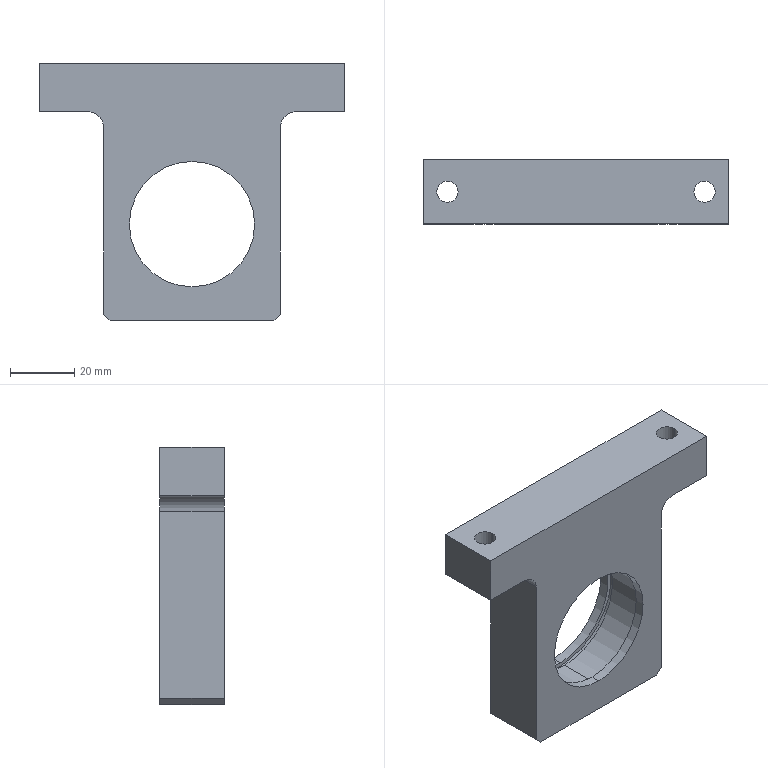Part | SolidWorks | features ICE 2, Chamfer 1, Extrusion 1, Fillet 1, HoleWzd 1 | 1 solid | 29 faces | box 95 x 20 x 80 mm | volume 71658 mm3 | plane 15 | cylinder 14 | commonest cylinder face diameters 6.6 x4 42 x4 10 x2 39 x2 44.5 x2
STEP:
#1=CARTESIAN_POINT('',(0.,16.85,-72.25));
#2=VERTEX_POINT('',#1);
#3=CARTESIAN_POINT('',(0.,16.85,-27.75));
#4=VERTEX_POINT('',#3);
#5=CARTESIAN_POINT('',(0.,16.85,-50.));
#6=DIRECTION('',(0.,1.,0.));
#7=DIRECTION('',(0.,0.,1.));
#8=AXIS2_PLACEMENT_3D('',#5,#6,#7);
#9=CIRCLE('',#8,22.25);
#10=EDGE_CURVE('',#2,#4,#9,.T.);
#11=ORIENTED_EDGE('',*,*,#10,.T.);
#12=CARTESIAN_POINT('',(0.,15.,-27.75));
#13=VERTEX_POINT('',#12);
#14=CARTESIAN_POINT('',(0.,16.85,-27.75));
#15=DIRECTION('',(0.,-1.,0.));
#16=VECTOR('',#15,1000.);
#17=LINE('',#14,#16);
#18=EDGE_CURVE('',#4,#13,#17,.T.);
#19=ORIENTED_EDGE('',*,*,#18,.T.);
#20=CARTESIAN_POINT('',(0.,15.,-72.25));
#21=VERTEX_POINT('',#20);
#22=CARTESIAN_POINT('',(0.,15.,-50.));
#23=DIRECTION('',(0.,1.,0.));
#24=DIRECTION('',(0.,0.,1.));
#25=AXIS2_PLACEMENT_3D('',#22,#23,#24);
#26=CIRCLE('',#25,22.25);
#27=EDGE_CURVE('',#21,#13,#26,.T.);
#28=ORIENTED_EDGE('',*,*,#27,.F.);
#29=CARTESIAN_POINT('',(0.,16.85,-72.25));
#30=DIRECTION('',(0.,-1.,0.));
#31=VECTOR('',#30,1000.);
#32=LINE('',#29,#31);
#33=EDGE_CURVE('',#2,#21,#32,.T.);
#34=ORIENTED_EDGE('',*,*,#33,.F.);
#35=EDGE_LOOP('',(#11,#19,#28,#34));
#36=FACE_OUTER_BOUND('',#35,.T.);
#37=CARTESIAN_POINT('',(0.,16.85,-50.));
#38=DIRECTION('',(0.,-1.,0.));
#39=DIRECTION('',(0.,0.,-1.));
#40=AXIS2_PLACEMENT_3D('',#37,#38,#39);
#41=CYLINDRICAL_SURFACE('',#40,22.25);
#42=ADVANCED_FACE('',(#36),#41,.F.);
#43=CARTESIAN_POINT('',(43.3,10.,0.));
#44=VERTEX_POINT('',#43);
#45=CARTESIAN_POINT('',(36.7,10.,0.));
#46=VERTEX_POINT('',#45);
#47=CARTESIAN_POINT('',(40.,10.,0.));
#48=DIRECTION('',(0.,0.,-1.));
#49=DIRECTION('',(-1.,0.,0.));
#50=AXIS2_PLACEMENT_3D('',#47,#48,#49);
#51=CIRCLE('',#50,3.3);
#52=EDGE_CURVE('',#44,#46,#51,.T.);
#53=ORIENTED_EDGE('',*,*,#52,.F.);
#54=CARTESIAN_POINT('',(43.3,10.,-15.));
#55=VERTEX_POINT('',#54);
#56=CARTESIAN_POINT('',(43.3,10.,-15.));
#57=DIRECTION('',(0.,0.,-1.));
#58=VECTOR('',#57,1000.);
#59=LINE('',#56,#58);
#60=EDGE_CURVE('',#44,#55,#59,.T.);
#61=ORIENTED_EDGE('',*,*,#60,.T.);
#62=CARTESIAN_POINT('',(36.7,10.,-15.));
#63=VERTEX_POINT('',#62);
#64=CARTESIAN_POINT('',(40.,10.,-15.));
#65=DIRECTION('',(0.,0.,-1.));
#66=DIRECTION('',(-1.,0.,0.));
#67=AXIS2_PLACEMENT_3D('',#64,#65,#66);
#68=CIRCLE('',#67,3.3);
#69=EDGE_CURVE('',#55,#63,#68,.T.);
#70=ORIENTED_EDGE('',*,*,#69,.T.);
#71=CARTESIAN_POINT('',(36.7,10.,-15.));
#72=DIRECTION('',(0.,0.,-1.));
#73=VECTOR('',#72,1000.);
#74=LINE('',#71,#73);
#75=EDGE_CURVE('',#46,#63,#74,.T.);
#76=ORIENTED_EDGE('',*,*,#75,.F.);
#77=EDGE_LOOP('',(#53,#61,#70,#76));
#78=FACE_OUTER_BOUND('',#77,.T.);
#79=CARTESIAN_POINT('',(40.,10.,-15.));
#80=DIRECTION('',(0.,0.,-1.));
#81=DIRECTION('',(-1.,0.,0.));
#82=AXIS2_PLACEMENT_3D('',#79,#80,#81);
#83=CYLINDRICAL_SURFACE('',#82,3.3);
#84=ADVANCED_FACE('',(#78),#83,.F.);
#85=CARTESIAN_POINT('',(-36.7,10.,0.));
#86=VERTEX_POINT('',#85);
#87=CARTESIAN_POINT('',(-43.3,10.,0.));
#88=VERTEX_POINT('',#87);
#89=CARTESIAN_POINT('',(-40.,10.,0.));
#90=DIRECTION('',(0.,0.,-1.));
#91=DIRECTION('',(-1.,0.,0.));
#92=AXIS2_PLACEMENT_3D('',#89,#90,#91);
#93=CIRCLE('',#92,3.3);
#94=EDGE_CURVE('',#86,#88,#93,.T.);
#95=ORIENTED_EDGE('',*,*,#94,.F.);
#96=CARTESIAN_POINT('',(-36.7,10.,-15.));
#97=VERTEX_POINT('',#96);
#98=CARTESIAN_POINT('',(-36.7,10.,-15.));
#99=DIRECTION('',(0.,0.,-1.));
#100=VECTOR('',#99,1000.);
#101=LINE('',#98,#100);
#102=EDGE_CURVE('',#86,#97,#101,.T.);
#103=ORIENTED_EDGE('',*,*,#102,.T.);
#104=CARTESIAN_POINT('',(-43.3,10.,-15.));
#105=VERTEX_POINT('',#104);
#106=CARTESIAN_POINT('',(-40.,10.,-15.));
#107=DIRECTION('',(0.,0.,-1.));
#108=DIRECTION('',(-1.,0.,0.));
#109=AXIS2_PLACEMENT_3D('',#106,#107,#108);
#110=CIRCLE('',#109,3.3);
#111=EDGE_CURVE('',#97,#105,#110,.T.);
#112=ORIENTED_EDGE('',*,*,#111,.T.);
#113=CARTESIAN_POINT('',(-43.3,10.,-15.));
#114=DIRECTION('',(0.,0.,-1.));
#115=VECTOR('',#114,1000.);
#116=LINE('',#113,#115);
#117=EDGE_CURVE('',#88,#105,#116,.T.);
#118=ORIENTED_EDGE('',*,*,#117,.F.);
#119=EDGE_LOOP('',(#95,#103,#112,#118));
#120=FACE_OUTER_BOUND('',#119,.T.);
#121=CARTESIAN_POINT('',(-40.,10.,-15.));
#122=DIRECTION('',(0.,0.,-1.));
#123=DIRECTION('',(-1.,0.,0.));
#124=AXIS2_PLACEMENT_3D('',#121,#122,#123);
#125=CYLINDRICAL_SURFACE('',#124,3.3);
#126=ADVANCED_FACE('',(#120),#125,.F.);
#127=CARTESIAN_POINT('',(0.,3.,-30.5));
#128=VERTEX_POINT('',#127);
#129=CARTESIAN_POINT('',(0.,3.,-69.5));
#130=VERTEX_POINT('',#129);
#131=CARTESIAN_POINT('',(0.,3.,-50.));
#132=DIRECTION('',(0.,-1.,0.));
#133=DIRECTION('',(0.,0.,-1.));
#134=AXIS2_PLACEMENT_3D('',#131,#132,#133);
#135=CIRCLE('',#134,19.5);
#136=EDGE_CURVE('',#128,#130,#135,.T.);
#137=ORIENTED_EDGE('',*,*,#136,.F.);
#138=CARTESIAN_POINT('',(0.,0.,-30.5));
#139=VERTEX_POINT('',#138);
#140=CARTESIAN_POINT('',(0.,3.,-30.5));
#141=DIRECTION('',(0.,-1.,0.));
#142=VECTOR('',#141,1000.);
#143=LINE('',#140,#142);
#144=EDGE_CURVE('',#128,#139,#143,.T.);
#145=ORIENTED_EDGE('',*,*,#144,.T.);
#146=CARTESIAN_POINT('',(0.,0.,-69.5));
#147=VERTEX_POINT('',#146);
#148=CARTESIAN_POINT('',(0.,0.,-50.));
#149=DIRECTION('',(0.,-1.,0.));
#150=DIRECTION('',(0.,0.,-1.));
#151=AXIS2_PLACEMENT_3D('',#148,#149,#150);
#152=CIRCLE('',#151,19.5);
#153=EDGE_CURVE('',#139,#147,#152,.T.);
#154=ORIENTED_EDGE('',*,*,#153,.T.);
#155=CARTESIAN_POINT('',(0.,3.,-69.5));
#156=DIRECTION('',(0.,-1.,0.));
#157=VECTOR('',#156,1000.);
#158=LINE('',#155,#157);
#159=EDGE_CURVE('',#130,#147,#158,.T.);
#160=ORIENTED_EDGE('',*,*,#159,.F.);
#161=EDGE_LOOP('',(#137,#145,#154,#160));
#162=FACE_OUTER_BOUND('',#161,.T.);
#163=CARTESIAN_POINT('',(0.,3.,-50.));
#164=DIRECTION('',(0.,-1.,0.));
#165=DIRECTION('',(0.,0.,-1.));
#166=AXIS2_PLACEMENT_3D('',#163,#164,#165);
#167=CYLINDRICAL_SURFACE('',#166,19.5);
#168=ADVANCED_FACE('',(#162),#167,.F.);
#169=CARTESIAN_POINT('',(0.,20.,-71.));
#170=VERTEX_POINT('',#169);
#171=CARTESIAN_POINT('',(0.,20.,-29.));
#172=VERTEX_POINT('',#171);
#173=CARTESIAN_POINT('',(0.,20.,-50.));
#174=DIRECTION('',(0.,1.,0.));
#175=DIRECTION('',(0.,0.,1.));
#176=AXIS2_PLACEMENT_3D('',#173,#174,#175);
#177=CIRCLE('',#176,21.);
#178=EDGE_CURVE('',#170,#172,#177,.T.);
#179=ORIENTED_EDGE('',*,*,#178,.T.);
#180=CARTESIAN_POINT('',(0.,16.85,-29.));
#181=VERTEX_POINT('',#180);
#182=CARTESIAN_POINT('',(0.,20.,-29.));
#183=DIRECTION('',(0.,-1.,0.));
#184=VECTOR('',#183,1000.);
#185=LINE('',#182,#184);
#186=EDGE_CURVE('',#172,#181,#185,.T.);
#187=ORIENTED_EDGE('',*,*,#186,.T.);
#188=CARTESIAN_POINT('',(0.,16.85,-71.));
#189=VERTEX_POINT('',#188);
#190=CARTESIAN_POINT('',(0.,16.85,-50.));
#191=DIRECTION('',(0.,1.,0.));
#192=DIRECTION('',(0.,0.,1.));
#193=AXIS2_PLACEMENT_3D('',#190,#191,#192);
#194=CIRCLE('',#193,21.);
#195=EDGE_CURVE('',#189,#181,#194,.T.);
#196=ORIENTED_EDGE('',*,*,#195,.F.);
#197=CARTESIAN_POINT('',(0.,20.,-71.));
#198=DIRECTION('',(0.,-1.,0.));
#199=VECTOR('',#198,1000.);
#200=LINE('',#197,#199);
#201=EDGE_CURVE('',#170,#189,#200,.T.);
#202=ORIENTED_EDGE('',*,*,#201,.F.);
#203=EDGE_LOOP('',(#179,#187,#196,#202));
#204=FACE_OUTER_BOUND('',#203,.T.);
#205=CARTESIAN_POINT('',(0.,20.,-50.));
#206=DIRECTION('',(0.,-1.,0.));
#207=DIRECTION('',(0.,0.,-1.));
#208=AXIS2_PLACEMENT_3D('',#205,#206,#207);
#209=CYLINDRICAL_SURFACE('',#208,21.);
#210=ADVANCED_FACE('',(#204),#209,.F.);
#211=CARTESIAN_POINT('',(0.,15.,-71.));
#212=VERTEX_POINT('',#211);
#213=CARTESIAN_POINT('',(0.,15.,-29.));
#214=VERTEX_POINT('',#213);
#215=CARTESIAN_POINT('',(0.,15.,-50.));
#216=DIRECTION('',(0.,1.,0.));
#217=DIRECTION('',(0.,0.,1.));
#218=AXIS2_PLACEMENT_3D('',#215,#216,#217);
#219=CIRCLE('',#218,21.);
#220=EDGE_CURVE('',#212,#214,#219,.T.);
#221=ORIENTED_EDGE('',*,*,#220,.T.);
#222=CARTESIAN_POINT('',(0.,3.,-29.));
#223=VERTEX_POINT('',#222);
#224=CARTESIAN_POINT('',(0.,20.,-29.));
#225=DIRECTION('',(0.,-1.,0.));
#226=VECTOR('',#225,1000.);
#227=LINE('',#224,#226);
#228=EDGE_CURVE('',#214,#223,#227,.T.);
#229=ORIENTED_EDGE('',*,*,#228,.T.);
#230=CARTESIAN_POINT('',(0.,3.,-71.));
#231=VERTEX_POINT('',#230);
#232=CARTESIAN_POINT('',(0.,3.,-50.));
#233=DIRECTION('',(0.,-1.,0.));
#234=DIRECTION('',(0.,0.,-1.));
#235=AXIS2_PLACEMENT_3D('',#232,#233,#234);
#236=CIRCLE('',#235,21.);
#237=EDGE_CURVE('',#223,#231,#236,.T.);
#238=ORIENTED_EDGE('',*,*,#237,.T.);
#239=CARTESIAN_POINT('',(0.,20.,-71.));
#240=DIRECTION('',(0.,-1.,0.));
#241=VECTOR('',#240,1000.);
#242=LINE('',#239,#241);
#243=EDGE_CURVE('',#212,#231,#242,.T.);
#244=ORIENTED_EDGE('',*,*,#243,.F.);
#245=EDGE_LOOP('',(#221,#229,#238,#244));
#246=FACE_OUTER_BOUND('',#245,.T.);
#247=CARTESIAN_POINT('',(0.,20.,-50.));
#248=DIRECTION('',(0.,-1.,0.));
#249=DIRECTION('',(0.,0.,-1.));
#250=AXIS2_PLACEMENT_3D('',#247,#248,#249);
#251=CYLINDRICAL_SURFACE('',#250,21.);
#252=ADVANCED_FACE('',(#246),#251,.F.);
#253=ORIENTED_EDGE('',*,*,#228,.F.);
#254=CARTESIAN_POINT('',(0.,15.,-50.));
#255=DIRECTION('',(0.,1.,0.));
#256=DIRECTION('',(0.,0.,1.));
#257=AXIS2_PLACEMENT_3D('',#254,#255,#256);
#258=CIRCLE('',#257,21.);
#259=EDGE_CURVE('',#214,#212,#258,.T.);
#260=ORIENTED_EDGE('',*,*,#259,.T.);
#261=ORIENTED_EDGE('',*,*,#243,.T.);
#262=CARTESIAN_POINT('',(0.,3.,-50.));
#263=DIRECTION('',(0.,-1.,0.));
#264=DIRECTION('',(0.,0.,-1.));
#265=AXIS2_PLACEMENT_3D('',#262,#263,#264);
#266=CIRCLE('',#265,21.);
#267=EDGE_CURVE('',#231,#223,#266,.T.);
#268=ORIENTED_EDGE('',*,*,#267,.T.);
#269=EDGE_LOOP('',(#253,#260,#261,#268));
#270=FACE_OUTER_BOUND('',#269,.T.);
#271=CARTESIAN_POINT('',(0.,20.,-50.));
#272=DIRECTION('',(0.,-1.,0.));
#273=DIRECTION('',(0.,0.,-1.));
#274=AXIS2_PLACEMENT_3D('',#271,#272,#273);
#275=CYLINDRICAL_SURFACE('',#274,21.);
#276=ADVANCED_FACE('',(#270),#275,.F.);
#277=ORIENTED_EDGE('',*,*,#186,.F.);
#278=CARTESIAN_POINT('',(0.,20.,-50.));
#279=DIRECTION('',(0.,1.,0.));
#280=DIRECTION('',(0.,0.,1.));
#281=AXIS2_PLACEMENT_3D('',#278,#279,#280);
#282=CIRCLE('',#281,21.);
#283=EDGE_CURVE('',#172,#170,#282,.T.);
#284=ORIENTED_EDGE('',*,*,#283,.T.);
#285=ORIENTED_EDGE('',*,*,#201,.T.);
#286=CARTESIAN_POINT('',(0.,16.85,-50.));
#287=DIRECTION('',(0.,1.,0.));
#288=DIRECTION('',(0.,0.,1.));
#289=AXIS2_PLACEMENT_3D('',#286,#287,#288);
#290=CIRCLE('',#289,21.);
#291=EDGE_CURVE('',#181,#189,#290,.T.);
#292=ORIENTED_EDGE('',*,*,#291,.F.);
#293=EDGE_LOOP('',(#277,#284,#285,#292));
#294=FACE_OUTER_BOUND('',#293,.T.);
#295=CARTESIAN_POINT('',(0.,20.,-50.));
#296=DIRECTION('',(0.,-1.,0.));
#297=DIRECTION('',(0.,0.,-1.));
#298=AXIS2_PLACEMENT_3D('',#295,#296,#297);
#299=CYLINDRICAL_SURFACE('',#298,21.);
#300=ADVANCED_FACE('',(#294),#299,.F.);
#301=CARTESIAN_POINT('',(47.5,20.,-15.));
#302=VERTEX_POINT('',#301);
#303=CARTESIAN_POINT('',(32.5,20.,-15.));
#304=VERTEX_POINT('',#303);
#305=CARTESIAN_POINT('',(27.5,20.,-15.));
#306=DIRECTION('',(-1.,0.,0.));
#307=VECTOR('',#306,1000.);
#308=LINE('',#305,#307);
#309=EDGE_CURVE('',#302,#304,#308,.T.);
#310=ORIENTED_EDGE('',*,*,#309,.T.);
#311=CARTESIAN_POINT('',(27.5,20.,-20.));
#312=VERTEX_POINT('',#311);
#313=CARTESIAN_POINT('',(32.5,20.,-20.));
#314=DIRECTION('',(0.,-1.,0.));
#315=DIRECTION('',(0.,0.,1.));
#316=AXIS2_PLACEMENT_3D('',#313,#314,#315);
#317=CIRCLE('',#316,5.);
#318=EDGE_CURVE('',#304,#312,#317,.T.);
#319=ORIENTED_EDGE('',*,*,#318,.T.);
#320=CARTESIAN_POINT('',(27.5,20.,-78.));
#321=VERTEX_POINT('',#320);
#322=CARTESIAN_POINT('',(27.5,20.,-80.));
#323=DIRECTION('',(0.,0.,-1.));
#324=VECTOR('',#323,1000.);
#325=LINE('',#322,#324);
#326=EDGE_CURVE('',#312,#321,#325,.T.);
#327=ORIENTED_EDGE('',*,*,#326,.T.);
#328=CARTESIAN_POINT('',(25.5,20.,-80.));
#329=VERTEX_POINT('',#328);
#330=CARTESIAN_POINT('',(52.75,20.,-52.75));
#331=DIRECTION('',(-0.7071,0.,-0.7071));
#332=VECTOR('',#331,1000.);
#333=LINE('',#330,#332);
#334=EDGE_CURVE('',#321,#329,#333,.T.);
#335=ORIENTED_EDGE('',*,*,#334,.T.);
#336=CARTESIAN_POINT('',(-25.5,20.,-80.));
#337=VERTEX_POINT('',#336);
#338=CARTESIAN_POINT('',(-27.5,20.,-80.));
#339=DIRECTION('',(-1.,0.,0.));
#340=VECTOR('',#339,1000.);
#341=LINE('',#338,#340);
#342=EDGE_CURVE('',#329,#337,#341,.T.);
#343=ORIENTED_EDGE('',*,*,#342,.T.);
#344=CARTESIAN_POINT('',(-27.5,20.,-78.));
#345=VERTEX_POINT('',#344);
#346=CARTESIAN_POINT('',(-52.75,20.,-52.75));
#347=DIRECTION('',(-0.7071,0.,0.7071));
#348=VECTOR('',#347,1000.);
#349=LINE('',#346,#348);
#350=EDGE_CURVE('',#337,#345,#349,.T.);
#351=ORIENTED_EDGE('',*,*,#350,.T.);
#352=CARTESIAN_POINT('',(-27.5,20.,-20.));
#353=VERTEX_POINT('',#352);
#354=CARTESIAN_POINT('',(-27.5,20.,-15.));
#355=DIRECTION('',(0.,0.,1.));
#356=VECTOR('',#355,1000.);
#357=LINE('',#354,#356);
#358=EDGE_CURVE('',#345,#353,#357,.T.);
#359=ORIENTED_EDGE('',*,*,#358,.T.);
#360=CARTESIAN_POINT('',(-32.5,20.,-15.));
#361=VERTEX_POINT('',#360);
#362=CARTESIAN_POINT('',(-32.5,20.,-20.));
#363=DIRECTION('',(0.,-1.,0.));
#364=DIRECTION('',(0.,0.,1.));
#365=AXIS2_PLACEMENT_3D('',#362,#363,#364);
#366=CIRCLE('',#365,5.);
#367=EDGE_CURVE('',#353,#361,#366,.T.);
#368=ORIENTED_EDGE('',*,*,#367,.T.);
#369=CARTESIAN_POINT('',(-47.5,20.,-15.));
#370=VERTEX_POINT('',#369);
#371=CARTESIAN_POINT('',(-47.5,20.,-15.));
#372=DIRECTION('',(-1.,0.,0.));
#373=VECTOR('',#372,1000.);
#374=LINE('',#371,#373);
#375=EDGE_CURVE('',#361,#370,#374,.T.);
#376=ORIENTED_EDGE('',*,*,#375,.T.);
#377=CARTESIAN_POINT('',(-47.5,20.,0.));
#378=VERTEX_POINT('',#377);
#379=CARTESIAN_POINT('',(-47.5,20.,0.));
#380=DIRECTION('',(0.,0.,1.));
#381=VECTOR('',#380,1000.);
#382=LINE('',#379,#381);
#383=EDGE_CURVE('',#370,#378,#382,.T.);
#384=ORIENTED_EDGE('',*,*,#383,.T.);
#385=CARTESIAN_POINT('',(47.5,20.,0.));
#386=VERTEX_POINT('',#385);
#387=CARTESIAN_POINT('',(-47.5,20.,0.));
#388=DIRECTION('',(1.,0.,0.));
#389=VECTOR('',#388,1000.);
#390=LINE('',#387,#389);
#391=EDGE_CURVE('',#378,#386,#390,.T.);
#392=ORIENTED_EDGE('',*,*,#391,.T.);
#393=CARTESIAN_POINT('',(47.5,20.,-15.));
#394=DIRECTION('',(0.,0.,-1.));
#395=VECTOR('',#394,1000.);
#396=LINE('',#393,#395);
#397=EDGE_CURVE('',#386,#302,#396,.T.);
#398=ORIENTED_EDGE('',*,*,#397,.T.);
#399=EDGE_LOOP('',(#310,#319,#327,#335,#343,#351,#359,#368,#376,#384,#392,#398));
#400=FACE_OUTER_BOUND('',#399,.T.);
#401=ORIENTED_EDGE('',*,*,#178,.F.);
#402=ORIENTED_EDGE('',*,*,#283,.F.);
#403=EDGE_LOOP('',(#401,#402));
#404=FACE_BOUND('',#403,.T.);
#405=CARTESIAN_POINT('',(0.,20.,0.));
#406=DIRECTION('',(0.,1.,0.));
#407=DIRECTION('',(0.,0.,1.));
#408=AXIS2_PLACEMENT_3D('',#405,#406,#407);
#409=PLANE('',#408);
#410=ADVANCED_FACE('',(#400,#404),#409,.T.);
#411=CARTESIAN_POINT('',(25.5,0.,-80.));
#412=VERTEX_POINT('',#411);
#413=CARTESIAN_POINT('',(-25.5,0.,-80.));
#414=VERTEX_POINT('',#413);
#415=CARTESIAN_POINT('',(-27.5,0.,-80.));
#416=DIRECTION('',(-1.,0.,0.));
#417=VECTOR('',#416,1000.);
#418=LINE('',#415,#417);
#419=EDGE_CURVE('',#412,#414,#418,.T.);
#420=ORIENTED_EDGE('',*,*,#419,.F.);
#421=CARTESIAN_POINT('',(27.5,0.,-78.));
#422=VERTEX_POINT('',#421);
#423=CARTESIAN_POINT('',(25.5,0.,-80.));
#424=DIRECTION('',(0.7071,0.,0.7071));
#425=VECTOR('',#424,1000.);
#426=LINE('',#423,#425);
#427=EDGE_CURVE('',#412,#422,#426,.T.);
#428=ORIENTED_EDGE('',*,*,#427,.T.);
#429=CARTESIAN_POINT('',(27.5,0.,-20.));
#430=VERTEX_POINT('',#429);
#431=CARTESIAN_POINT('',(27.5,0.,-80.));
#432=DIRECTION('',(0.,0.,-1.));
#433=VECTOR('',#432,1000.);
#434=LINE('',#431,#433);
#435=EDGE_CURVE('',#430,#422,#434,.T.);
#436=ORIENTED_EDGE('',*,*,#435,.F.);
#437=CARTESIAN_POINT('',(32.5,0.,-15.));
#438=VERTEX_POINT('',#437);
#439=CARTESIAN_POINT('',(32.5,0.,-20.));
#440=DIRECTION('',(0.,1.,0.));
#441=DIRECTION('',(0.,0.,1.));
#442=AXIS2_PLACEMENT_3D('',#439,#440,#441);
#443=CIRCLE('',#442,5.);
#444=EDGE_CURVE('',#430,#438,#443,.T.);
#445=ORIENTED_EDGE('',*,*,#444,.T.);
#446=CARTESIAN_POINT('',(47.5,0.,-15.));
#447=VERTEX_POINT('',#446);
#448=CARTESIAN_POINT('',(27.5,0.,-15.));
#449=DIRECTION('',(-1.,0.,0.));
#450=VECTOR('',#449,1000.);
#451=LINE('',#448,#450);
#452=EDGE_CURVE('',#447,#438,#451,.T.);
#453=ORIENTED_EDGE('',*,*,#452,.F.);
#454=CARTESIAN_POINT('',(47.5,0.,0.));
#455=VERTEX_POINT('',#454);
#456=CARTESIAN_POINT('',(47.5,0.,-15.));
#457=DIRECTION('',(0.,0.,-1.));
#458=VECTOR('',#457,1000.);
#459=LINE('',#456,#458);
#460=EDGE_CURVE('',#455,#447,#459,.T.);
#461=ORIENTED_EDGE('',*,*,#460,.F.);
#462=CARTESIAN_POINT('',(-47.5,0.,0.));
#463=VERTEX_POINT('',#462);
#464=CARTESIAN_POINT('',(-47.5,0.,0.));
#465=DIRECTION('',(1.,0.,0.));
#466=VECTOR('',#465,1000.);
#467=LINE('',#464,#466);
#468=EDGE_CURVE('',#463,#455,#467,.T.);
#469=ORIENTED_EDGE('',*,*,#468,.F.);
#470=CARTESIAN_POINT('',(-47.5,0.,-15.));
#471=VERTEX_POINT('',#470);
#472=CARTESIAN_POINT('',(-47.5,0.,0.));
#473=DIRECTION('',(0.,0.,1.));
#474=VECTOR('',#473,1000.);
#475=LINE('',#472,#474);
#476=EDGE_CURVE('',#471,#463,#475,.T.);
#477=ORIENTED_EDGE('',*,*,#476,.F.);
#478=CARTESIAN_POINT('',(-32.5,0.,-15.));
#479=VERTEX_POINT('',#478);
#480=CARTESIAN_POINT('',(-47.5,0.,-15.));
#481=DIRECTION('',(-1.,0.,0.));
#482=VECTOR('',#481,1000.);
#483=LINE('',#480,#482);
#484=EDGE_CURVE('',#479,#471,#483,.T.);
#485=ORIENTED_EDGE('',*,*,#484,.F.);
#486=CARTESIAN_POINT('',(-27.5,0.,-20.));
#487=VERTEX_POINT('',#486);
#488=CARTESIAN_POINT('',(-32.5,0.,-20.));
#489=DIRECTION('',(0.,1.,0.));
#490=DIRECTION('',(0.,0.,1.));
#491=AXIS2_PLACEMENT_3D('',#488,#489,#490);
#492=CIRCLE('',#491,5.);
#493=EDGE_CURVE('',#479,#487,#492,.T.);
#494=ORIENTED_EDGE('',*,*,#493,.T.);
#495=CARTESIAN_POINT('',(-27.5,0.,-78.));
#496=VERTEX_POINT('',#495);
#497=CARTESIAN_POINT('',(-27.5,0.,-15.));
#498=DIRECTION('',(0.,0.,1.));
#499=VECTOR('',#498,1000.);
#500=LINE('',#497,#499);
#501=EDGE_CURVE('',#496,#487,#500,.T.);
#502=ORIENTED_EDGE('',*,*,#501,.F.);
#503=CARTESIAN_POINT('',(-27.5,0.,-78.));
#504=DIRECTION('',(0.7071,0.,-0.7071));
#505=VECTOR('',#504,1000.);
#506=LINE('',#503,#505);
#507=EDGE_CURVE('',#496,#414,#506,.T.);
#508=ORIENTED_EDGE('',*,*,#507,.T.);
#509=EDGE_LOOP('',(#420,#428,#436,#445,#453,#461,#469,#477,#485,#494,#502,#508));
#510=FACE_OUTER_BOUND('',#509,.T.);
#511=CARTESIAN_POINT('',(0.,0.,-50.));
#512=DIRECTION('',(0.,-1.,0.));
#513=DIRECTION('',(0.,0.,-1.));
#514=AXIS2_PLACEMENT_3D('',#511,#512,#513);
#515=CIRCLE('',#514,19.5);
#516=EDGE_CURVE('',#147,#139,#515,.T.);
#517=ORIENTED_EDGE('',*,*,#516,.F.);
#518=ORIENTED_EDGE('',*,*,#153,.F.);
#519=EDGE_LOOP('',(#517,#518));
#520=FACE_BOUND('',#519,.T.);
#521=CARTESIAN_POINT('',(0.,0.,0.));
#522=DIRECTION('',(0.,1.,0.));
#523=DIRECTION('',(0.,0.,1.));
#524=AXIS2_PLACEMENT_3D('',#521,#522,#523);
#525=PLANE('',#524);
#526=ADVANCED_FACE('',(#510,#520),#525,.F.);
#527=ORIENTED_EDGE('',*,*,#460,.T.);
#528=CARTESIAN_POINT('',(47.5,20.,-15.));
#529=DIRECTION('',(0.,-1.,0.));
#530=VECTOR('',#529,1000.);
#531=LINE('',#528,#530);
#532=EDGE_CURVE('',#302,#447,#531,.T.);
#533=ORIENTED_EDGE('',*,*,#532,.F.);
#534=ORIENTED_EDGE('',*,*,#397,.F.);
#535=CARTESIAN_POINT('',(47.5,20.,0.));
#536=DIRECTION('',(0.,-1.,0.));
#537=VECTOR('',#536,1000.);
#538=LINE('',#535,#537);
#539=EDGE_CURVE('',#386,#455,#538,.T.);
#540=ORIENTED_EDGE('',*,*,#539,.T.);
#541=EDGE_LOOP('',(#527,#533,#534,#540));
#542=FACE_OUTER_BOUND('',#541,.T.);
#543=CARTESIAN_POINT('',(47.5,20.,-15.));
#544=DIRECTION('',(-1.,0.,0.));
#545=DIRECTION('',(0.,0.,1.));
#546=AXIS2_PLACEMENT_3D('',#543,#544,#545);
#547=PLANE('',#546);
#548=ADVANCED_FACE('',(#542),#547,.F.);
#549=CARTESIAN_POINT('',(40.,10.,-15.));
#550=DIRECTION('',(0.,0.,-1.));
#551=DIRECTION('',(-1.,0.,0.));
#552=AXIS2_PLACEMENT_3D('',#549,#550,#551);
#553=CIRCLE('',#552,3.3);
#554=EDGE_CURVE('',#63,#55,#553,.T.);
#555=ORIENTED_EDGE('',*,*,#554,.F.);
#556=ORIENTED_EDGE('',*,*,#69,.F.);
#557=EDGE_LOOP('',(#555,#556));
#558=FACE_BOUND('',#557,.T.);
#559=ORIENTED_EDGE('',*,*,#452,.T.);
#560=CARTESIAN_POINT('',(32.5,20.,-15.));
#561=DIRECTION('',(0.,1.,0.));
#562=VECTOR('',#561,1000.);
#563=LINE('',#560,#562);
#564=EDGE_CURVE('',#438,#304,#563,.T.);
#565=ORIENTED_EDGE('',*,*,#564,.T.);
#566=ORIENTED_EDGE('',*,*,#309,.F.);
#567=ORIENTED_EDGE('',*,*,#532,.T.);
#568=EDGE_LOOP('',(#559,#565,#566,#567));
#569=FACE_OUTER_BOUND('',#568,.T.);
#570=CARTESIAN_POINT('',(27.5,20.,-15.));
#571=DIRECTION('',(0.,0.,1.));
#572=DIRECTION('',(1.,0.,0.));
#573=AXIS2_PLACEMENT_3D('',#570,#571,#572);
#574=PLANE('',#573);
#575=ADVANCED_FACE('',(#558,#569),#574,.F.);
#576=ORIENTED_EDGE('',*,*,#326,.F.);
#577=CARTESIAN_POINT('',(27.5,0.,-20.));
#578=DIRECTION('',(0.,-1.,0.));
#579=VECTOR('',#578,1000.);
#580=LINE('',#577,#579);
#581=EDGE_CURVE('',#312,#430,#580,.T.);
#582=ORIENTED_EDGE('',*,*,#581,.T.);
#583=ORIENTED_EDGE('',*,*,#435,.T.);
#584=CARTESIAN_POINT('',(27.5,20.,-78.));
#585=DIRECTION('',(0.,1.,0.));
#586=VECTOR('',#585,1000.);
#587=LINE('',#584,#586);
#588=EDGE_CURVE('',#422,#321,#587,.T.);
#589=ORIENTED_EDGE('',*,*,#588,.T.);
#590=EDGE_LOOP('',(#576,#582,#583,#589));
#591=FACE_OUTER_BOUND('',#590,.T.);
#592=CARTESIAN_POINT('',(27.5,20.,-80.));
#593=DIRECTION('',(-1.,0.,0.));
#594=DIRECTION('',(0.,0.,1.));
#595=AXIS2_PLACEMENT_3D('',#592,#593,#594);
#596=PLANE('',#595);
#597=ADVANCED_FACE('',(#591),#596,.F.);
#598=ORIENTED_EDGE('',*,*,#342,.F.);
#599=CARTESIAN_POINT('',(25.5,20.,-80.));
#600=DIRECTION('',(0.,-1.,0.));
#601=VECTOR('',#600,1000.);
#602=LINE('',#599,#601);
#603=EDGE_CURVE('',#329,#412,#602,.T.);
#604=ORIENTED_EDGE('',*,*,#603,.T.);
#605=ORIENTED_EDGE('',*,*,#419,.T.);
#606=CARTESIAN_POINT('',(-25.5,20.,-80.));
#607=DIRECTION('',(0.,1.,0.));
#608=VECTOR('',#607,1000.);
#609=LINE('',#606,#608);
#610=EDGE_CURVE('',#414,#337,#609,.T.);
#611=ORIENTED_EDGE('',*,*,#610,.T.);
#612=EDGE_LOOP('',(#598,#604,#605,#611));
#613=FACE_OUTER_BOUND('',#612,.T.);
#614=CARTESIAN_POINT('',(-27.5,20.,-80.));
#615=DIRECTION('',(0.,0.,1.));
#616=DIRECTION('',(1.,0.,0.));
#617=AXIS2_PLACEMENT_3D('',#614,#615,#616);
#618=PLANE('',#617);
#619=ADVANCED_FACE('',(#613),#618,.F.);
#620=ORIENTED_EDGE('',*,*,#501,.T.);
#621=CARTESIAN_POINT('',(-27.5,20.,-20.));
#622=DIRECTION('',(0.,1.,0.));
#623=VECTOR('',#622,1000.);
#624=LINE('',#621,#623);
#625=EDGE_CURVE('',#487,#353,#624,.T.);
#626=ORIENTED_EDGE('',*,*,#625,.T.);
#627=ORIENTED_EDGE('',*,*,#358,.F.);
#628=CARTESIAN_POINT('',(-27.5,20.,-78.));
#629=DIRECTION('',(0.,-1.,0.));
#630=VECTOR('',#629,1000.);
#631=LINE('',#628,#630);
#632=EDGE_CURVE('',#345,#496,#631,.T.);
#633=ORIENTED_EDGE('',*,*,#632,.T.);
#634=EDGE_LOOP('',(#620,#626,#627,#633));
#635=FACE_OUTER_BOUND('',#634,.T.);
#636=CARTESIAN_POINT('',(-27.5,20.,-15.));
#637=DIRECTION('',(1.,0.,0.));
#638=DIRECTION('',(0.,0.,-1.));
#639=AXIS2_PLACEMENT_3D('',#636,#637,#638);
#640=PLANE('',#639);
#641=ADVANCED_FACE('',(#635),#640,.F.);
#642=CARTESIAN_POINT('',(-40.,10.,-15.));
#643=DIRECTION('',(0.,0.,-1.));
#644=DIRECTION('',(-1.,0.,0.));
#645=AXIS2_PLACEMENT_3D('',#642,#643,#644);
#646=CIRCLE('',#645,3.3);
#647=EDGE_CURVE('',#105,#97,#646,.T.);
#648=ORIENTED_EDGE('',*,*,#647,.F.);
#649=ORIENTED_EDGE('',*,*,#111,.F.);
#650=EDGE_LOOP('',(#648,#649));
#651=FACE_BOUND('',#650,.T.);
#652=ORIENTED_EDGE('',*,*,#375,.F.);
#653=CARTESIAN_POINT('',(-32.5,0.,-15.));
#654=DIRECTION('',(0.,-1.,0.));
#655=VECTOR('',#654,1000.);
#656=LINE('',#653,#655);
#657=EDGE_CURVE('',#361,#479,#656,.T.);
#658=ORIENTED_EDGE('',*,*,#657,.T.);
#659=ORIENTED_EDGE('',*,*,#484,.T.);
#660=CARTESIAN_POINT('',(-47.5,20.,-15.));
#661=DIRECTION('',(0.,-1.,0.));
#662=VECTOR('',#661,1000.);
#663=LINE('',#660,#662);
#664=EDGE_CURVE('',#370,#471,#663,.T.);
#665=ORIENTED_EDGE('',*,*,#664,.F.);
#666=EDGE_LOOP('',(#652,#658,#659,#665));
#667=FACE_OUTER_BOUND('',#666,.T.);
#668=CARTESIAN_POINT('',(-47.5,20.,-15.));
#669=DIRECTION('',(0.,0.,1.));
#670=DIRECTION('',(1.,0.,0.));
#671=AXIS2_PLACEMENT_3D('',#668,#669,#670);
#672=PLANE('',#671);
#673=ADVANCED_FACE('',(#651,#667),#672,.F.);
#674=ORIENTED_EDGE('',*,*,#476,.T.);
#675=CARTESIAN_POINT('',(-47.5,20.,0.));
#676=DIRECTION('',(0.,-1.,0.));
#677=VECTOR('',#676,1000.);
#678=LINE('',#675,#677);
#679=EDGE_CURVE('',#378,#463,#678,.T.);
#680=ORIENTED_EDGE('',*,*,#679,.F.);
#681=ORIENTED_EDGE('',*,*,#383,.F.);
#682=ORIENTED_EDGE('',*,*,#664,.T.);
#683=EDGE_LOOP('',(#674,#680,#681,#682));
#684=FACE_OUTER_BOUND('',#683,.T.);
#685=CARTESIAN_POINT('',(-47.5,20.,0.));
#686=DIRECTION('',(1.,0.,0.));
#687=DIRECTION('',(0.,0.,-1.));
#688=AXIS2_PLACEMENT_3D('',#685,#686,#687);
#689=PLANE('',#688);
#690=ADVANCED_FACE('',(#684),#689,.F.);
#691=CARTESIAN_POINT('',(40.,10.,0.));
#692=DIRECTION('',(0.,0.,-1.));
#693=DIRECTION('',(-1.,0.,0.));
#694=AXIS2_PLACEMENT_3D('',#691,#692,#693);
#695=CIRCLE('',#694,3.3);
#696=EDGE_CURVE('',#46,#44,#695,.T.);
#697=ORIENTED_EDGE('',*,*,#696,.T.);
#698=ORIENTED_EDGE('',*,*,#52,.T.);
#699=EDGE_LOOP('',(#697,#698));
#700=FACE_BOUND('',#699,.T.);
#701=CARTESIAN_POINT('',(-40.,10.,0.));
#702=DIRECTION('',(0.,0.,-1.));
#703=DIRECTION('',(-1.,0.,0.));
#704=AXIS2_PLACEMENT_3D('',#701,#702,#703);
#705=CIRCLE('',#704,3.3);
#706=EDGE_CURVE('',#88,#86,#705,.T.);
#707=ORIENTED_EDGE('',*,*,#706,.T.);
#708=ORIENTED_EDGE('',*,*,#94,.T.);
#709=EDGE_LOOP('',(#707,#708));
#710=FACE_BOUND('',#709,.T.);
#711=ORIENTED_EDGE('',*,*,#468,.T.);
#712=ORIENTED_EDGE('',*,*,#539,.F.);
#713=ORIENTED_EDGE('',*,*,#391,.F.);
#714=ORIENTED_EDGE('',*,*,#679,.T.);
#715=EDGE_LOOP('',(#711,#712,#713,#714));
#716=FACE_OUTER_BOUND('',#715,.T.);
#717=CARTESIAN_POINT('',(-47.5,20.,0.));
#718=DIRECTION('',(0.,0.,-1.));
#719=DIRECTION('',(-1.,0.,0.));
#720=AXIS2_PLACEMENT_3D('',#717,#718,#719);
#721=PLANE('',#720);
#722=ADVANCED_FACE('',(#700,#710,#716),#721,.F.);
#723=ORIENTED_EDGE('',*,*,#334,.F.);
#724=ORIENTED_EDGE('',*,*,#588,.F.);
#725=ORIENTED_EDGE('',*,*,#427,.F.);
#726=ORIENTED_EDGE('',*,*,#603,.F.);
#727=EDGE_LOOP('',(#723,#724,#725,#726));
#728=FACE_OUTER_BOUND('',#727,.T.);
#729=CARTESIAN_POINT('',(25.5,20.,-80.));
#730=DIRECTION('',(-0.7071,0.,0.7071));
#731=DIRECTION('',(0.,-1.,0.));
#732=AXIS2_PLACEMENT_3D('',#729,#730,#731);
#733=PLANE('',#732);
#734=ADVANCED_FACE('',(#728),#733,.F.);
#735=ORIENTED_EDGE('',*,*,#350,.F.);
#736=ORIENTED_EDGE('',*,*,#610,.F.);
#737=ORIENTED_EDGE('',*,*,#507,.F.);
#738=ORIENTED_EDGE('',*,*,#632,.F.);
#739=EDGE_LOOP('',(#735,#736,#737,#738));
#740=FACE_OUTER_BOUND('',#739,.T.);
#741=CARTESIAN_POINT('',(-27.5,20.,-78.));
#742=DIRECTION('',(0.7071,0.,0.7071));
#743=DIRECTION('',(0.,-1.,0.));
#744=AXIS2_PLACEMENT_3D('',#741,#742,#743);
#745=PLANE('',#744);
#746=ADVANCED_FACE('',(#740),#745,.F.);
#747=ORIENTED_EDGE('',*,*,#318,.F.);
#748=ORIENTED_EDGE('',*,*,#564,.F.);
#749=ORIENTED_EDGE('',*,*,#444,.F.);
#750=ORIENTED_EDGE('',*,*,#581,.F.);
#751=EDGE_LOOP('',(#747,#748,#749,#750));
#752=FACE_OUTER_BOUND('',#751,.T.);
#753=CARTESIAN_POINT('',(32.5,20.,-20.));
#754=DIRECTION('',(0.,1.,0.));
#755=DIRECTION('',(0.,0.,1.));
#756=AXIS2_PLACEMENT_3D('',#753,#754,#755);
#757=CYLINDRICAL_SURFACE('',#756,5.);
#758=ADVANCED_FACE('',(#752),#757,.F.);
#759=ORIENTED_EDGE('',*,*,#367,.F.);
#760=ORIENTED_EDGE('',*,*,#625,.F.);
#761=ORIENTED_EDGE('',*,*,#493,.F.);
#762=ORIENTED_EDGE('',*,*,#657,.F.);
#763=EDGE_LOOP('',(#759,#760,#761,#762));
#764=FACE_OUTER_BOUND('',#763,.T.);
#765=CARTESIAN_POINT('',(-32.5,20.,-20.));
#766=DIRECTION('',(0.,1.,0.));
#767=DIRECTION('',(0.,0.,1.));
#768=AXIS2_PLACEMENT_3D('',#765,#766,#767);
#769=CYLINDRICAL_SURFACE('',#768,5.);
#770=ADVANCED_FACE('',(#764),#769,.F.);
#771=CARTESIAN_POINT('',(0.,3.,-50.));
#772=DIRECTION('',(0.,-1.,0.));
#773=DIRECTION('',(0.,0.,-1.));
#774=AXIS2_PLACEMENT_3D('',#771,#772,#773);
#775=CIRCLE('',#774,19.5);
#776=EDGE_CURVE('',#130,#128,#775,.T.);
#777=ORIENTED_EDGE('',*,*,#776,.T.);
#778=ORIENTED_EDGE('',*,*,#136,.T.);
#779=EDGE_LOOP('',(#777,#778));
#780=FACE_BOUND('',#779,.T.);
#781=ORIENTED_EDGE('',*,*,#267,.F.);
#782=ORIENTED_EDGE('',*,*,#237,.F.);
#783=EDGE_LOOP('',(#781,#782));
#784=FACE_OUTER_BOUND('',#783,.T.);
#785=CARTESIAN_POINT('',(0.,3.,-50.));
#786=DIRECTION('',(0.,-1.,0.));
#787=DIRECTION('',(0.,0.,-1.));
#788=AXIS2_PLACEMENT_3D('',#785,#786,#787);
#789=PLANE('',#788);
#790=ADVANCED_FACE('',(#780,#784),#789,.F.);
#791=ORIENTED_EDGE('',*,*,#144,.F.);
#792=ORIENTED_EDGE('',*,*,#776,.F.);
#793=ORIENTED_EDGE('',*,*,#159,.T.);
#794=ORIENTED_EDGE('',*,*,#516,.T.);
#795=EDGE_LOOP('',(#791,#792,#793,#794));
#796=FACE_OUTER_BOUND('',#795,.T.);
#797=CARTESIAN_POINT('',(0.,3.,-50.));
#798=DIRECTION('',(0.,-1.,0.));
#799=DIRECTION('',(0.,0.,-1.));
#800=AXIS2_PLACEMENT_3D('',#797,#798,#799);
#801=CYLINDRICAL_SURFACE('',#800,19.5);
#802=ADVANCED_FACE('',(#796),#801,.F.);
#803=ORIENTED_EDGE('',*,*,#102,.F.);
#804=ORIENTED_EDGE('',*,*,#706,.F.);
#805=ORIENTED_EDGE('',*,*,#117,.T.);
#806=ORIENTED_EDGE('',*,*,#647,.T.);
#807=EDGE_LOOP('',(#803,#804,#805,#806));
#808=FACE_OUTER_BOUND('',#807,.T.);
#809=CARTESIAN_POINT('',(-40.,10.,-15.));
#810=DIRECTION('',(0.,0.,-1.));
#811=DIRECTION('',(-1.,0.,0.));
#812=AXIS2_PLACEMENT_3D('',#809,#810,#811);
#813=CYLINDRICAL_SURFACE('',#812,3.3);
#814=ADVANCED_FACE('',(#808),#813,.F.);
#815=ORIENTED_EDGE('',*,*,#60,.F.);
#816=ORIENTED_EDGE('',*,*,#696,.F.);
#817=ORIENTED_EDGE('',*,*,#75,.T.);
#818=ORIENTED_EDGE('',*,*,#554,.T.);
#819=EDGE_LOOP('',(#815,#816,#817,#818));
#820=FACE_OUTER_BOUND('',#819,.T.);
#821=CARTESIAN_POINT('',(40.,10.,-15.));
#822=DIRECTION('',(0.,0.,-1.));
#823=DIRECTION('',(-1.,0.,0.));
#824=AXIS2_PLACEMENT_3D('',#821,#822,#823);
#825=CYLINDRICAL_SURFACE('',#824,3.3);
#826=ADVANCED_FACE('',(#820),#825,.F.);
#827=ORIENTED_EDGE('',*,*,#10,.F.);
#828=CARTESIAN_POINT('',(0.,16.85,-50.));
#829=DIRECTION('',(0.,1.,0.));
#830=DIRECTION('',(0.,0.,1.));
#831=AXIS2_PLACEMENT_3D('',#828,#829,#830);
#832=CIRCLE('',#831,22.25);
#833=EDGE_CURVE('',#4,#2,#832,.T.);
#834=ORIENTED_EDGE('',*,*,#833,.F.);
#835=EDGE_LOOP('',(#827,#834));
#836=FACE_OUTER_BOUND('',#835,.T.);
#837=ORIENTED_EDGE('',*,*,#195,.T.);
#838=ORIENTED_EDGE('',*,*,#291,.T.);
#839=EDGE_LOOP('',(#837,#838));
#840=FACE_BOUND('',#839,.T.);
#841=CARTESIAN_POINT('',(0.,16.85,-50.));
#842=DIRECTION('',(0.,1.,0.));
#843=DIRECTION('',(0.,0.,1.));
#844=AXIS2_PLACEMENT_3D('',#841,#842,#843);
#845=PLANE('',#844);
#846=ADVANCED_FACE('',(#836,#840),#845,.F.);
#847=ORIENTED_EDGE('',*,*,#27,.T.);
#848=CARTESIAN_POINT('',(0.,15.,-50.));
#849=DIRECTION('',(0.,1.,0.));
#850=DIRECTION('',(0.,0.,1.));
#851=AXIS2_PLACEMENT_3D('',#848,#849,#850);
#852=CIRCLE('',#851,22.25);
#853=EDGE_CURVE('',#13,#21,#852,.T.);
#854=ORIENTED_EDGE('',*,*,#853,.T.);
#855=EDGE_LOOP('',(#847,#854));
#856=FACE_OUTER_BOUND('',#855,.T.);
#857=ORIENTED_EDGE('',*,*,#220,.F.);
#858=ORIENTED_EDGE('',*,*,#259,.F.);
#859=EDGE_LOOP('',(#857,#858));
#860=FACE_BOUND('',#859,.T.);
#861=CARTESIAN_POINT('',(0.,15.,-50.));
#862=DIRECTION('',(0.,1.,0.));
#863=DIRECTION('',(0.,0.,1.));
#864=AXIS2_PLACEMENT_3D('',#861,#862,#863);
#865=PLANE('',#864);
#866=ADVANCED_FACE('',(#856,#860),#865,.T.);
#867=ORIENTED_EDGE('',*,*,#18,.F.);
#868=ORIENTED_EDGE('',*,*,#833,.T.);
#869=ORIENTED_EDGE('',*,*,#33,.T.);
#870=ORIENTED_EDGE('',*,*,#853,.F.);
#871=EDGE_LOOP('',(#867,#868,#869,#870));
#872=FACE_OUTER_BOUND('',#871,.T.);
#873=CARTESIAN_POINT('',(0.,16.85,-50.));
#874=DIRECTION('',(0.,-1.,0.));
#875=DIRECTION('',(0.,0.,-1.));
#876=AXIS2_PLACEMENT_3D('',#873,#874,#875);
#877=CYLINDRICAL_SURFACE('',#876,22.25);
#878=ADVANCED_FACE('',(#872),#877,.F.);
#879=CLOSED_SHELL('',(#42,#84,#126,#168,#210,#252,#276,#300,#410,#526,#548,#575,#597,#619,#641,#673,#690,#722,#734,#746,#758,#770,#790,#802,#814,#826,#846,#866,#878));
#880=MANIFOLD_SOLID_BREP('',#879);
#881=CARTESIAN_POINT('',(0.,0.,0.));
#882=DIRECTION('',(0.,0.,1.));
#883=DIRECTION('',(1.,0.,0.));
#884=AXIS2_PLACEMENT_3D('',#881,#882,#883);
#885=(LENGTH_UNIT()NAMED_UNIT(*)SI_UNIT(.MILLI.,.METRE.));
#886=UNCERTAINTY_MEASURE_WITH_UNIT(LENGTH_MEASURE(0.00001),#885,'','');
#887=(NAMED_UNIT(*)PLANE_ANGLE_UNIT()SI_UNIT($,.RADIAN.));
#888=(NAMED_UNIT(*)SI_UNIT($,.STERADIAN.)SOLID_ANGLE_UNIT());
#889=(GEOMETRIC_REPRESENTATION_CONTEXT(3)GLOBAL_UNCERTAINTY_ASSIGNED_CONTEXT((#886))GLOBAL_UNIT_ASSIGNED_CONTEXT((#885,#887,#888))REPRESENTATION_CONTEXT('',''));
#890=ADVANCED_BREP_SHAPE_REPRESENTATION('',(#880,#884),#889);